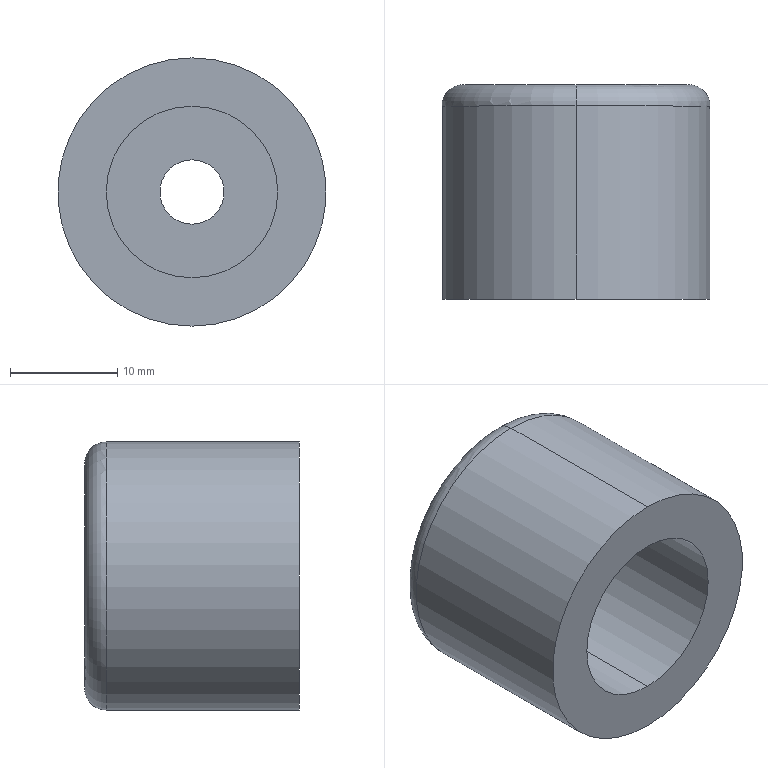Part | SolidWorks | features BaseBody 1 | 1 solid | 11 faces | box 25 x 20 x 25 mm | volume 7114 mm3 | cylinder 6 | plane 3 | torus 2 | commonest cylinder face diameters 6 x2 16 x2 25 x2
STEP:
#1=CARTESIAN_POINT('',(0.,18.,-12.5));
#2=VERTEX_POINT('',#1);
#3=CARTESIAN_POINT('',(0.,18.,12.5));
#4=VERTEX_POINT('',#3);
#5=CARTESIAN_POINT('',(0.,18.,0.));
#6=DIRECTION('',(0.,-1.,0.));
#7=DIRECTION('',(0.,0.,1.));
#8=AXIS2_PLACEMENT_3D('',#5,#6,#7);
#9=CIRCLE('',#8,12.5);
#10=EDGE_CURVE('',#2,#4,#9,.T.);
#11=ORIENTED_EDGE('',*,*,#10,.F.);
#12=CARTESIAN_POINT('',(0.,20.,-10.5));
#13=VERTEX_POINT('',#12);
#14=CARTESIAN_POINT('',(0.,18.,-10.5));
#15=DIRECTION('',(1.,0.,0.));
#16=DIRECTION('',(0.,0.,-1.));
#17=AXIS2_PLACEMENT_3D('',#14,#15,#16);
#18=CIRCLE('',#17,2.);
#19=EDGE_CURVE('',#2,#13,#18,.T.);
#20=ORIENTED_EDGE('',*,*,#19,.T.);
#21=CARTESIAN_POINT('',(0.,20.,10.5));
#22=VERTEX_POINT('',#21);
#23=CARTESIAN_POINT('',(0.,20.,0.));
#24=DIRECTION('',(0.,1.,0.));
#25=DIRECTION('',(0.,0.,1.));
#26=AXIS2_PLACEMENT_3D('',#23,#24,#25);
#27=CIRCLE('',#26,10.5);
#28=EDGE_CURVE('',#22,#13,#27,.T.);
#29=ORIENTED_EDGE('',*,*,#28,.F.);
#30=CARTESIAN_POINT('',(0.,18.,10.5));
#31=DIRECTION('',(-1.,0.,0.));
#32=DIRECTION('',(0.,0.,1.));
#33=AXIS2_PLACEMENT_3D('',#30,#31,#32);
#34=CIRCLE('',#33,2.);
#35=EDGE_CURVE('',#4,#22,#34,.T.);
#36=ORIENTED_EDGE('',*,*,#35,.F.);
#37=EDGE_LOOP('',(#11,#20,#29,#36));
#38=FACE_OUTER_BOUND('',#37,.T.);
#39=CARTESIAN_POINT('',(0.,18.,0.));
#40=DIRECTION('',(0.,1.,0.));
#41=DIRECTION('',(0.,0.,1.));
#42=AXIS2_PLACEMENT_3D('',#39,#40,#41);
#43=TOROIDAL_SURFACE('',#42,10.5,2.);
#44=ADVANCED_FACE('',(#38),#43,.T.);
#45=CARTESIAN_POINT('',(0.,20.,3.));
#46=VERTEX_POINT('',#45);
#47=CARTESIAN_POINT('',(0.,20.,-3.));
#48=VERTEX_POINT('',#47);
#49=CARTESIAN_POINT('',(0.,20.,0.));
#50=DIRECTION('',(0.,-1.,0.));
#51=DIRECTION('',(0.,0.,-1.));
#52=AXIS2_PLACEMENT_3D('',#49,#50,#51);
#53=CIRCLE('',#52,3.);
#54=EDGE_CURVE('',#46,#48,#53,.T.);
#55=ORIENTED_EDGE('',*,*,#54,.F.);
#56=CARTESIAN_POINT('',(0.,12.,3.));
#57=VERTEX_POINT('',#56);
#58=CARTESIAN_POINT('',(0.,20.,3.));
#59=DIRECTION('',(0.,-1.,0.));
#60=VECTOR('',#59,1000.);
#61=LINE('',#58,#60);
#62=EDGE_CURVE('',#46,#57,#61,.T.);
#63=ORIENTED_EDGE('',*,*,#62,.T.);
#64=CARTESIAN_POINT('',(0.,12.,-3.));
#65=VERTEX_POINT('',#64);
#66=CARTESIAN_POINT('',(0.,12.,0.));
#67=DIRECTION('',(0.,-1.,0.));
#68=DIRECTION('',(0.,0.,-1.));
#69=AXIS2_PLACEMENT_3D('',#66,#67,#68);
#70=CIRCLE('',#69,3.);
#71=EDGE_CURVE('',#57,#65,#70,.T.);
#72=ORIENTED_EDGE('',*,*,#71,.T.);
#73=CARTESIAN_POINT('',(0.,20.,-3.));
#74=DIRECTION('',(0.,-1.,0.));
#75=VECTOR('',#74,1000.);
#76=LINE('',#73,#75);
#77=EDGE_CURVE('',#48,#65,#76,.T.);
#78=ORIENTED_EDGE('',*,*,#77,.F.);
#79=EDGE_LOOP('',(#55,#63,#72,#78));
#80=FACE_OUTER_BOUND('',#79,.T.);
#81=CARTESIAN_POINT('',(0.,20.,0.));
#82=DIRECTION('',(0.,-1.,0.));
#83=DIRECTION('',(0.,0.,-1.));
#84=AXIS2_PLACEMENT_3D('',#81,#82,#83);
#85=CYLINDRICAL_SURFACE('',#84,3.);
#86=ADVANCED_FACE('',(#80),#85,.F.);
#87=CARTESIAN_POINT('',(0.,12.,8.));
#88=VERTEX_POINT('',#87);
#89=CARTESIAN_POINT('',(0.,12.,-8.));
#90=VERTEX_POINT('',#89);
#91=CARTESIAN_POINT('',(0.,12.,0.));
#92=DIRECTION('',(0.,-1.,0.));
#93=DIRECTION('',(0.,0.,-1.));
#94=AXIS2_PLACEMENT_3D('',#91,#92,#93);
#95=CIRCLE('',#94,8.);
#96=EDGE_CURVE('',#88,#90,#95,.T.);
#97=ORIENTED_EDGE('',*,*,#96,.F.);
#98=CARTESIAN_POINT('',(0.,0.,8.));
#99=VERTEX_POINT('',#98);
#100=CARTESIAN_POINT('',(0.,12.,8.));
#101=DIRECTION('',(0.,-1.,0.));
#102=VECTOR('',#101,1000.);
#103=LINE('',#100,#102);
#104=EDGE_CURVE('',#88,#99,#103,.T.);
#105=ORIENTED_EDGE('',*,*,#104,.T.);
#106=CARTESIAN_POINT('',(0.,0.,-8.));
#107=VERTEX_POINT('',#106);
#108=CARTESIAN_POINT('',(0.,0.,0.));
#109=DIRECTION('',(0.,-1.,0.));
#110=DIRECTION('',(0.,0.,-1.));
#111=AXIS2_PLACEMENT_3D('',#108,#109,#110);
#112=CIRCLE('',#111,8.);
#113=EDGE_CURVE('',#99,#107,#112,.T.);
#114=ORIENTED_EDGE('',*,*,#113,.T.);
#115=CARTESIAN_POINT('',(0.,12.,-8.));
#116=DIRECTION('',(0.,-1.,0.));
#117=VECTOR('',#116,1000.);
#118=LINE('',#115,#117);
#119=EDGE_CURVE('',#90,#107,#118,.T.);
#120=ORIENTED_EDGE('',*,*,#119,.F.);
#121=EDGE_LOOP('',(#97,#105,#114,#120));
#122=FACE_OUTER_BOUND('',#121,.T.);
#123=CARTESIAN_POINT('',(0.,12.,0.));
#124=DIRECTION('',(0.,-1.,0.));
#125=DIRECTION('',(0.,0.,-1.));
#126=AXIS2_PLACEMENT_3D('',#123,#124,#125);
#127=CYLINDRICAL_SURFACE('',#126,8.);
#128=ADVANCED_FACE('',(#122),#127,.F.);
#129=ORIENTED_EDGE('',*,*,#10,.T.);
#130=CARTESIAN_POINT('',(0.,0.,12.5));
#131=VERTEX_POINT('',#130);
#132=CARTESIAN_POINT('',(0.,20.,12.5));
#133=DIRECTION('',(0.,-1.,0.));
#134=VECTOR('',#133,1000.);
#135=LINE('',#132,#134);
#136=EDGE_CURVE('',#4,#131,#135,.T.);
#137=ORIENTED_EDGE('',*,*,#136,.T.);
#138=CARTESIAN_POINT('',(0.,0.,-12.5));
#139=VERTEX_POINT('',#138);
#140=CARTESIAN_POINT('',(0.,0.,0.));
#141=DIRECTION('',(0.,1.,0.));
#142=DIRECTION('',(0.,0.,1.));
#143=AXIS2_PLACEMENT_3D('',#140,#141,#142);
#144=CIRCLE('',#143,12.5);
#145=EDGE_CURVE('',#131,#139,#144,.T.);
#146=ORIENTED_EDGE('',*,*,#145,.T.);
#147=CARTESIAN_POINT('',(0.,20.,-12.5));
#148=DIRECTION('',(0.,-1.,0.));
#149=VECTOR('',#148,1000.);
#150=LINE('',#147,#149);
#151=EDGE_CURVE('',#2,#139,#150,.T.);
#152=ORIENTED_EDGE('',*,*,#151,.F.);
#153=EDGE_LOOP('',(#129,#137,#146,#152));
#154=FACE_OUTER_BOUND('',#153,.T.);
#155=CARTESIAN_POINT('',(0.,20.,0.));
#156=DIRECTION('',(0.,-1.,0.));
#157=DIRECTION('',(0.,0.,-1.));
#158=AXIS2_PLACEMENT_3D('',#155,#156,#157);
#159=CYLINDRICAL_SURFACE('',#158,12.5);
#160=ADVANCED_FACE('',(#154),#159,.T.);
#161=CARTESIAN_POINT('',(0.,12.,0.));
#162=DIRECTION('',(0.,-1.,0.));
#163=DIRECTION('',(0.,0.,-1.));
#164=AXIS2_PLACEMENT_3D('',#161,#162,#163);
#165=CIRCLE('',#164,3.);
#166=EDGE_CURVE('',#65,#57,#165,.T.);
#167=ORIENTED_EDGE('',*,*,#166,.F.);
#168=ORIENTED_EDGE('',*,*,#71,.F.);
#169=EDGE_LOOP('',(#167,#168));
#170=FACE_BOUND('',#169,.T.);
#171=CARTESIAN_POINT('',(0.,12.,0.));
#172=DIRECTION('',(0.,-1.,0.));
#173=DIRECTION('',(0.,0.,-1.));
#174=AXIS2_PLACEMENT_3D('',#171,#172,#173);
#175=CIRCLE('',#174,8.);
#176=EDGE_CURVE('',#90,#88,#175,.T.);
#177=ORIENTED_EDGE('',*,*,#176,.T.);
#178=ORIENTED_EDGE('',*,*,#96,.T.);
#179=EDGE_LOOP('',(#177,#178));
#180=FACE_OUTER_BOUND('',#179,.T.);
#181=CARTESIAN_POINT('',(0.,12.,0.));
#182=DIRECTION('',(0.,-1.,0.));
#183=DIRECTION('',(0.,0.,-1.));
#184=AXIS2_PLACEMENT_3D('',#181,#182,#183);
#185=PLANE('',#184);
#186=ADVANCED_FACE('',(#170,#180),#185,.T.);
#187=CARTESIAN_POINT('',(0.,0.,0.));
#188=DIRECTION('',(0.,-1.,0.));
#189=DIRECTION('',(0.,0.,-1.));
#190=AXIS2_PLACEMENT_3D('',#187,#188,#189);
#191=CIRCLE('',#190,8.);
#192=EDGE_CURVE('',#107,#99,#191,.T.);
#193=ORIENTED_EDGE('',*,*,#192,.F.);
#194=ORIENTED_EDGE('',*,*,#113,.F.);
#195=EDGE_LOOP('',(#193,#194));
#196=FACE_BOUND('',#195,.T.);
#197=CARTESIAN_POINT('',(0.,0.,0.));
#198=DIRECTION('',(0.,1.,0.));
#199=DIRECTION('',(0.,0.,1.));
#200=AXIS2_PLACEMENT_3D('',#197,#198,#199);
#201=CIRCLE('',#200,12.5);
#202=EDGE_CURVE('',#139,#131,#201,.T.);
#203=ORIENTED_EDGE('',*,*,#202,.F.);
#204=ORIENTED_EDGE('',*,*,#145,.F.);
#205=EDGE_LOOP('',(#203,#204));
#206=FACE_OUTER_BOUND('',#205,.T.);
#207=CARTESIAN_POINT('',(0.,0.,0.));
#208=DIRECTION('',(0.,1.,0.));
#209=DIRECTION('',(1.,0.,0.));
#210=AXIS2_PLACEMENT_3D('',#207,#208,#209);
#211=PLANE('',#210);
#212=ADVANCED_FACE('',(#196,#206),#211,.F.);
#213=CARTESIAN_POINT('',(0.,20.,0.));
#214=DIRECTION('',(0.,-1.,0.));
#215=DIRECTION('',(0.,0.,-1.));
#216=AXIS2_PLACEMENT_3D('',#213,#214,#215);
#217=CIRCLE('',#216,3.);
#218=EDGE_CURVE('',#48,#46,#217,.T.);
#219=ORIENTED_EDGE('',*,*,#218,.T.);
#220=ORIENTED_EDGE('',*,*,#54,.T.);
#221=EDGE_LOOP('',(#219,#220));
#222=FACE_BOUND('',#221,.T.);
#223=ORIENTED_EDGE('',*,*,#28,.T.);
#224=CARTESIAN_POINT('',(0.,20.,0.));
#225=DIRECTION('',(0.,1.,0.));
#226=DIRECTION('',(0.,0.,1.));
#227=AXIS2_PLACEMENT_3D('',#224,#225,#226);
#228=CIRCLE('',#227,10.5);
#229=EDGE_CURVE('',#13,#22,#228,.T.);
#230=ORIENTED_EDGE('',*,*,#229,.T.);
#231=EDGE_LOOP('',(#223,#230));
#232=FACE_OUTER_BOUND('',#231,.T.);
#233=CARTESIAN_POINT('',(0.,20.,0.));
#234=DIRECTION('',(0.,1.,0.));
#235=DIRECTION('',(1.,0.,0.));
#236=AXIS2_PLACEMENT_3D('',#233,#234,#235);
#237=PLANE('',#236);
#238=ADVANCED_FACE('',(#222,#232),#237,.T.);
#239=ORIENTED_EDGE('',*,*,#136,.F.);
#240=CARTESIAN_POINT('',(0.,18.,0.));
#241=DIRECTION('',(0.,-1.,0.));
#242=DIRECTION('',(0.,0.,1.));
#243=AXIS2_PLACEMENT_3D('',#240,#241,#242);
#244=CIRCLE('',#243,12.5);
#245=EDGE_CURVE('',#4,#2,#244,.T.);
#246=ORIENTED_EDGE('',*,*,#245,.T.);
#247=ORIENTED_EDGE('',*,*,#151,.T.);
#248=ORIENTED_EDGE('',*,*,#202,.T.);
#249=EDGE_LOOP('',(#239,#246,#247,#248));
#250=FACE_OUTER_BOUND('',#249,.T.);
#251=CARTESIAN_POINT('',(0.,20.,0.));
#252=DIRECTION('',(0.,-1.,0.));
#253=DIRECTION('',(0.,0.,-1.));
#254=AXIS2_PLACEMENT_3D('',#251,#252,#253);
#255=CYLINDRICAL_SURFACE('',#254,12.5);
#256=ADVANCED_FACE('',(#250),#255,.T.);
#257=ORIENTED_EDGE('',*,*,#104,.F.);
#258=ORIENTED_EDGE('',*,*,#176,.F.);
#259=ORIENTED_EDGE('',*,*,#119,.T.);
#260=ORIENTED_EDGE('',*,*,#192,.T.);
#261=EDGE_LOOP('',(#257,#258,#259,#260));
#262=FACE_OUTER_BOUND('',#261,.T.);
#263=CARTESIAN_POINT('',(0.,12.,0.));
#264=DIRECTION('',(0.,-1.,0.));
#265=DIRECTION('',(0.,0.,-1.));
#266=AXIS2_PLACEMENT_3D('',#263,#264,#265);
#267=CYLINDRICAL_SURFACE('',#266,8.);
#268=ADVANCED_FACE('',(#262),#267,.F.);
#269=ORIENTED_EDGE('',*,*,#62,.F.);
#270=ORIENTED_EDGE('',*,*,#218,.F.);
#271=ORIENTED_EDGE('',*,*,#77,.T.);
#272=ORIENTED_EDGE('',*,*,#166,.T.);
#273=EDGE_LOOP('',(#269,#270,#271,#272));
#274=FACE_OUTER_BOUND('',#273,.T.);
#275=CARTESIAN_POINT('',(0.,20.,0.));
#276=DIRECTION('',(0.,-1.,0.));
#277=DIRECTION('',(0.,0.,-1.));
#278=AXIS2_PLACEMENT_3D('',#275,#276,#277);
#279=CYLINDRICAL_SURFACE('',#278,3.);
#280=ADVANCED_FACE('',(#274),#279,.F.);
#281=ORIENTED_EDGE('',*,*,#19,.F.);
#282=ORIENTED_EDGE('',*,*,#245,.F.);
#283=ORIENTED_EDGE('',*,*,#35,.T.);
#284=ORIENTED_EDGE('',*,*,#229,.F.);
#285=EDGE_LOOP('',(#281,#282,#283,#284));
#286=FACE_OUTER_BOUND('',#285,.T.);
#287=CARTESIAN_POINT('',(0.,18.,0.));
#288=DIRECTION('',(0.,1.,0.));
#289=DIRECTION('',(0.,0.,1.));
#290=AXIS2_PLACEMENT_3D('',#287,#288,#289);
#291=TOROIDAL_SURFACE('',#290,10.5,2.);
#292=ADVANCED_FACE('',(#286),#291,.T.);
#293=CLOSED_SHELL('',(#44,#86,#128,#160,#186,#212,#238,#256,#268,#280,#292));
#294=MANIFOLD_SOLID_BREP('',#293);
#295=CARTESIAN_POINT('',(0.,0.,0.));
#296=DIRECTION('',(0.,0.,1.));
#297=DIRECTION('',(1.,0.,0.));
#298=AXIS2_PLACEMENT_3D('',#295,#296,#297);
#299=(LENGTH_UNIT()NAMED_UNIT(*)SI_UNIT(.MILLI.,.METRE.));
#300=UNCERTAINTY_MEASURE_WITH_UNIT(LENGTH_MEASURE(0.00001),#299,'','');
#301=(NAMED_UNIT(*)PLANE_ANGLE_UNIT()SI_UNIT($,.RADIAN.));
#302=(NAMED_UNIT(*)SI_UNIT($,.STERADIAN.)SOLID_ANGLE_UNIT());
#303=(GEOMETRIC_REPRESENTATION_CONTEXT(3)GLOBAL_UNCERTAINTY_ASSIGNED_CONTEXT((#300))GLOBAL_UNIT_ASSIGNED_CONTEXT((#299,#301,#302))REPRESENTATION_CONTEXT('',''));
#304=ADVANCED_BREP_SHAPE_REPRESENTATION('',(#294,#298),#303);